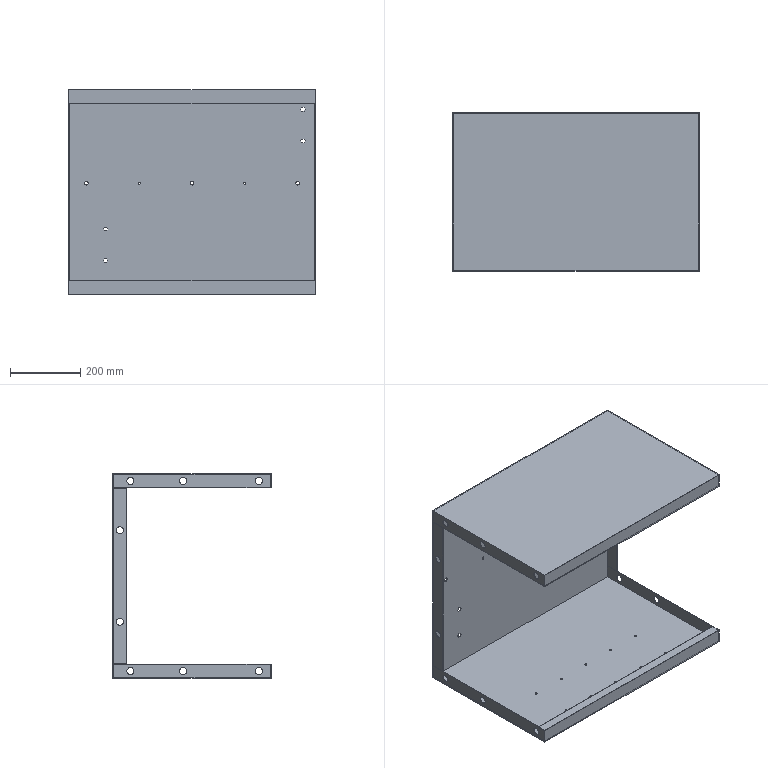Part | SolidWorks | features BaseBody 1 | 1 solid | 132 faces | box 700 x 450 x 580 mm | volume 2436073 mm3 | plane 70 | cylinder 62 | commonest cylinder face diameters 20 x32 5.5 x20 10.5 x6 6.5 x4